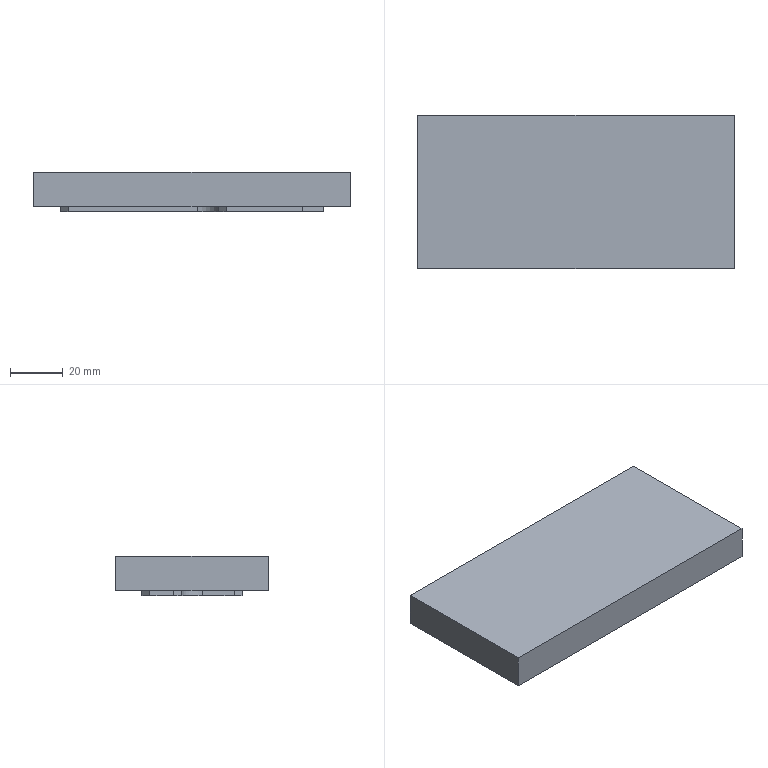NC program | NX | posted with a generic post | part box 120 x 58 x 15 mm
Whole program:
N10 G17 G21 G94 G90
(ZLEVEL_PROFILE_1_COPY_COPY , TOOL : D10)
N12 T04 M6
N14 G54
N16 G17 G0 G90 X59.051 Y7.28 S9500 M3
N18 G43 Z30. H4
N20 Z2.
N22 G94 G1 X58.6 Y7.401 F2000.
N24 G3 X57.635 Y7.141 R1.
N26 G1 X53.748 Y3.252
N28 X50.748 Y0.252
N30 G2 X47. Y-1.3 R5.3
N32 G1 X-2.
N34 G3 X-4.7 Y-4. R2.7
N36 G1 Y-15.383
N38 X-4.723 Y-15.503
N40 G2 X-6.252 Y-19.748 R5.3
N42 G1 X-9.252 Y-22.748
N44 G2 X-13. Y-24.3 R5.3
N46 G1 X-42.
N48 G2 X-45.748 Y-22.748 R5.3
N50 G1 X-53.748 Y-14.748
N52 G2 X-53.967 Y-14.515 R5.3
N54 G1 X-53.983 Y-14.512
N56 X-57.345 Y-11.149
N58 G3 X-58.311 Y-10.89 R1.
N60 G1 X-58.822 Y-11.027
N62 G0 Z1.
N64 G1 X-58.311 Y-10.89
N66 G2 X-57.345 Y-11.149 R1.
N68 G1 X-53.983 Y-14.512
N70 X-53.967 Y-14.515
N72 G3 X-53.748 Y-14.748 R5.3
N74 G1 X-45.748 Y-22.748
N76 G3 X-42. Y-24.3 R5.3
N78 G1 X-13.
N80 G3 X-9.252 Y-22.748 R5.3
N82 G1 X-6.252 Y-19.748
N84 G3 X-4.723 Y-15.503 R5.3
N86 G1 X-4.7 Y-15.383
N88 Y-4.
N90 G2 X-2. Y-1.3 R2.7
N92 G1 X47.
N94 G3 X50.748 Y0.252 R5.3
N96 G1 X53.748 Y3.252
N98 X57.635 Y7.141
N100 G2 X58.6 Y7.401 R1.
N102 G1 X59.051 Y7.28
N104 G0 Z0.
N106 G1 X58.6 Y7.401
N108 G3 X57.635 Y7.141 R1.
N110 G1 X53.748 Y3.252
N112 X50.748 Y0.252
N114 G2 X47. Y-1.3 R5.3
N116 G1 X-2.
N118 G3 X-4.7 Y-4. R2.7
N120 G1 Y-15.383
N122 X-4.723 Y-15.503
N124 G2 X-6.252 Y-19.748 R5.3
N126 G1 X-9.252 Y-22.748
N128 G2 X-13. Y-24.3 R5.3
N130 G1 X-42.
N132 G2 X-45.748 Y-22.748 R5.3
N134 G1 X-53.748 Y-14.748
N136 G2 X-53.967 Y-14.515 R5.3
N138 G1 X-53.983 Y-14.512
N140 X-57.345 Y-11.149
N142 G3 X-58.311 Y-10.89 R1.
N144 G1 X-58.822 Y-11.027
N146 G0 Z-1.
N148 G1 X-58.311 Y-10.89
N150 G2 X-57.345 Y-11.149 R1.
N152 G1 X-53.983 Y-14.512
N154 X-53.967 Y-14.515
N156 G3 X-53.748 Y-14.748 R5.3
N158 G1 X-45.748 Y-22.748
N160 G3 X-42. Y-24.3 R5.3
N162 G1 X-13.
N164 G3 X-9.252 Y-22.748 R5.3
N166 G1 X-6.252 Y-19.748
N168 G3 X-4.723 Y-15.503 R5.3
N170 G1 X-4.7 Y-15.383
N172 Y-4.
N174 G2 X-2. Y-1.3 R2.7
N176 G1 X47.
N178 G3 X50.748 Y0.252 R5.3
N180 G1 X53.748 Y3.252
N182 X57.635 Y7.141
N184 G2 X58.6 Y7.401 R1.
N186 G1 X59.051 Y7.28
N188 G0 Z30.
N190 M5
(FLOOR_WALL_COPY_COPY , TOOL : D63)
N192 T03 M6
N194 G54
N196 G17 G0 G90 X-84.499 Y0. S6500 M3
N198 G43 Z30. H3
N200 Z5.
N202 G94 G1 Z2. F1250.
N204 X-81.499
N206 X81.499
N208 X84.499
N210 Z5.
N212 G0 Z30.
N214 X-84.499
N216 Z4.
N218 G1 Z1.
N220 X-81.499
N222 X81.499
N224 X84.499
N226 Z4.
N228 G0 Z30.
N230 X-84.499
N232 Z3.
N234 G1 Z0.
N236 X-81.499
N238 X81.499
N240 X84.499
N242 Z3.
N244 G0 Z30.
N246 M5
(11_COPY_COPY_COPY , TOOL : D6A45)
N248 T01 M6
N250 G54
N252 G17 G0 G90 X-30. Y0.741 S9500 M3
N254 G43 Z30. H1
N256 Z3.
N258 G94 G1 Z-1. F1000.
N260 G3 X-30.741 Y0. R0.741
N262 X-30. Y0.741 R-0.741
N264 X-30.52 Y0.441 R0.6
N266 G1 Z2.
N268 G0 Z30.
N270 X-30. Y14.791
N272 Z3.
N274 G1 Z-1.
N276 G3 X-44.791 Y0. R14.791
N278 X-30. Y-14.791 R14.791
N280 X-29.209 Y-14. R0.791
N282 X-30. Y-13.209 R0.791
N284 G2 X-43.209 Y0. R13.209
N286 X-30. Y13.209 R13.209
N288 G3 X-29.209 Y14. R0.791
N290 X-30. Y14.791 R0.791
N292 X-30.52 Y14.491 R0.6
N294 G1 Z2.
N296 G0 Z30.
N298 X44.042 Y13.081
N300 Z2.
N302 G1 Z-1.
N304 X44.52 Y13.991
N306 G3 X44. Y14.291 R0.6
N308 G1 X-6.
N310 G3 X-7.291 Y13. R1.291
N312 X-6. Y11.709 R1.291
N314 G1 X44.
N316 G3 X45.291 Y13. R1.291
N318 X44. Y14.291 R1.291
N320 X43.48 Y13.991 R0.6
N322 G1 X42.961 Y13.091
N324 Z2.
N326 G0 Z30.
N328 X-42.921 Y20.952
N330 Z2.
N332 G1 Z-1.
N334 X-42.52 Y20.259
N336 G3 X-42.001 Y19.959 R0.6
N338 G1 X47.001
N340 G2 X47.677 Y19.678 R0.957
N342 G1 X50.678 Y16.677
N344 G2 X50.959 Y16.001 R0.957
N346 G1 Y6.999
N348 G2 X50.678 Y6.323 R0.957
N350 G1 X47.677 Y3.322
N352 G2 X47.001 Y3.041 R0.957
N354 G1 X-2.
N356 G3 X-9.041 Y-4. R7.041
N358 G1 Y-16.001
N360 G2 X-9.322 Y-16.677 R0.957
N362 G1 X-12.323 Y-19.678
N364 G2 X-12.999 Y-19.959 R0.957
N366 G1 X-42.001
N368 G2 X-42.677 Y-19.678 R0.957
N370 G1 X-50.678 Y-11.677
N372 G2 X-50.959 Y-11. R0.957
N374 G1 Y11.
N376 G2 X-50.678 Y11.677 R0.957
N378 G1 X-42.677 Y19.678
N380 G2 X-42.001 Y19.959 R0.957
N382 G3 X-41.481 Y20.259 R0.6
N384 G1 X-40.961 Y21.159
N386 Z2.
N388 G0 Z30.
N390 M5
N392 M2